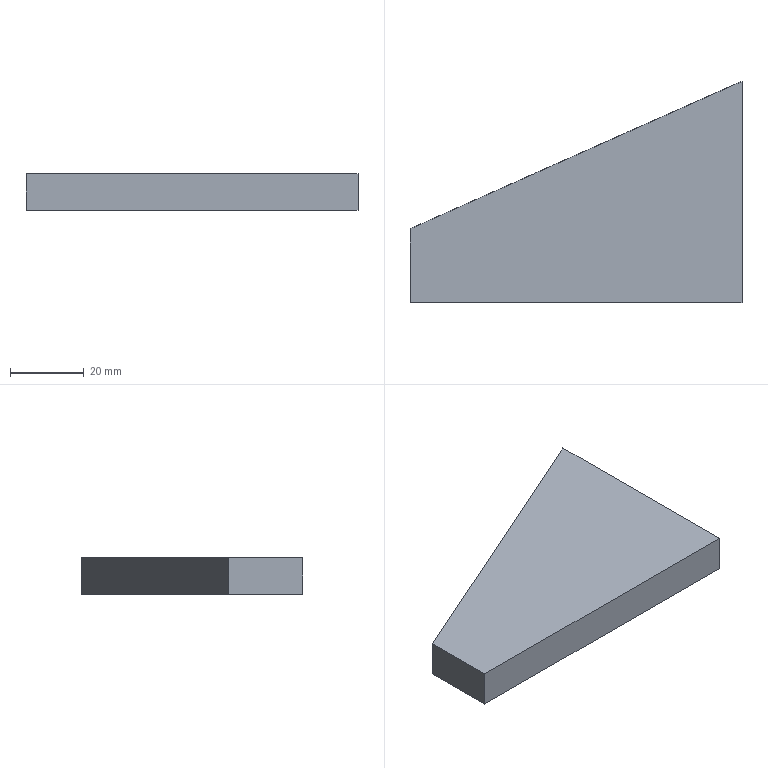Part | SolidWorks | features BaseBody 1, ICE 1 | 1 solid | 6 faces | box 90 x 60 x 10 mm | volume 36000 mm3 | plane 6
STEP:
#1=CARTESIAN_POINT('',(-25.,10.,1240.));
#2=VERTEX_POINT('',#1);
#3=CARTESIAN_POINT('',(-25.,-50.,1240.));
#4=VERTEX_POINT('',#3);
#5=CARTESIAN_POINT('',(-25.,-15.,1240.));
#6=DIRECTION('',(0.,-1.,0.));
#7=VECTOR('',#6,1000.);
#8=LINE('',#5,#7);
#9=EDGE_CURVE('',#2,#4,#8,.T.);
#10=ORIENTED_EDGE('',*,*,#9,.F.);
#11=CARTESIAN_POINT('',(-115.,-30.,1240.));
#12=VERTEX_POINT('',#11);
#13=CARTESIAN_POINT('',(-25.,10.,1240.));
#14=DIRECTION('',(-0.9138,-0.4061,0.));
#15=VECTOR('',#14,1000.);
#16=LINE('',#13,#15);
#17=EDGE_CURVE('',#2,#12,#16,.T.);
#18=ORIENTED_EDGE('',*,*,#17,.T.);
#19=CARTESIAN_POINT('',(-115.,-50.,1240.));
#20=VERTEX_POINT('',#19);
#21=CARTESIAN_POINT('',(-115.,-15.,1240.));
#22=DIRECTION('',(0.,1.,0.));
#23=VECTOR('',#22,1000.);
#24=LINE('',#21,#23);
#25=EDGE_CURVE('',#20,#12,#24,.T.);
#26=ORIENTED_EDGE('',*,*,#25,.F.);
#27=CARTESIAN_POINT('',(-70.,-50.,1240.));
#28=DIRECTION('',(-1.,0.,0.));
#29=VECTOR('',#28,1000.);
#30=LINE('',#27,#29);
#31=EDGE_CURVE('',#4,#20,#30,.T.);
#32=ORIENTED_EDGE('',*,*,#31,.F.);
#33=EDGE_LOOP('',(#10,#18,#26,#32));
#34=FACE_OUTER_BOUND('',#33,.T.);
#35=CARTESIAN_POINT('',(-23.2,-51.4,1240.));
#36=DIRECTION('',(0.,0.,-1.));
#37=DIRECTION('',(-1.,0.,0.));
#38=AXIS2_PLACEMENT_3D('',#35,#36,#37);
#39=PLANE('',#38);
#40=ADVANCED_FACE('',(#34),#39,.F.);
#41=CARTESIAN_POINT('',(-25.,10.,1230.));
#42=VERTEX_POINT('',#41);
#43=CARTESIAN_POINT('',(-25.,10.,1240.));
#44=DIRECTION('',(0.,0.,-1.));
#45=VECTOR('',#44,1000.);
#46=LINE('',#43,#45);
#47=EDGE_CURVE('',#2,#42,#46,.T.);
#48=ORIENTED_EDGE('',*,*,#47,.F.);
#49=ORIENTED_EDGE('',*,*,#9,.T.);
#50=CARTESIAN_POINT('',(-25.,-50.,1230.));
#51=VERTEX_POINT('',#50);
#52=CARTESIAN_POINT('',(-25.,-50.,1235.));
#53=DIRECTION('',(0.,0.,-1.));
#54=VECTOR('',#53,1000.);
#55=LINE('',#52,#54);
#56=EDGE_CURVE('',#4,#51,#55,.T.);
#57=ORIENTED_EDGE('',*,*,#56,.T.);
#58=CARTESIAN_POINT('',(-25.,-15.,1230.));
#59=DIRECTION('',(0.,1.,0.));
#60=VECTOR('',#59,1000.);
#61=LINE('',#58,#60);
#62=EDGE_CURVE('',#51,#42,#61,.T.);
#63=ORIENTED_EDGE('',*,*,#62,.T.);
#64=EDGE_LOOP('',(#48,#49,#57,#63));
#65=FACE_OUTER_BOUND('',#64,.T.);
#66=CARTESIAN_POINT('',(-25.,21.4,1241.145));
#67=DIRECTION('',(1.,0.,0.));
#68=DIRECTION('',(0.,-1.,0.));
#69=AXIS2_PLACEMENT_3D('',#66,#67,#68);
#70=PLANE('',#69);
#71=ADVANCED_FACE('',(#65),#70,.T.);
#72=CARTESIAN_POINT('',(-115.,-30.,1230.));
#73=VERTEX_POINT('',#72);
#74=CARTESIAN_POINT('',(-115.,-50.,1230.));
#75=VERTEX_POINT('',#74);
#76=CARTESIAN_POINT('',(-115.,-40.,1230.));
#77=DIRECTION('',(0.,-1.,0.));
#78=VECTOR('',#77,1000.);
#79=LINE('',#76,#78);
#80=EDGE_CURVE('',#73,#75,#79,.T.);
#81=ORIENTED_EDGE('',*,*,#80,.T.);
#82=CARTESIAN_POINT('',(-115.,-50.,1235.));
#83=DIRECTION('',(0.,0.,1.));
#84=VECTOR('',#83,1000.);
#85=LINE('',#82,#84);
#86=EDGE_CURVE('',#75,#20,#85,.T.);
#87=ORIENTED_EDGE('',*,*,#86,.T.);
#88=ORIENTED_EDGE('',*,*,#25,.T.);
#89=CARTESIAN_POINT('',(-115.,-30.,1235.));
#90=DIRECTION('',(0.,0.,1.));
#91=VECTOR('',#90,1000.);
#92=LINE('',#89,#91);
#93=EDGE_CURVE('',#73,#12,#92,.T.);
#94=ORIENTED_EDGE('',*,*,#93,.F.);
#95=EDGE_LOOP('',(#81,#87,#88,#94));
#96=FACE_OUTER_BOUND('',#95,.T.);
#97=CARTESIAN_POINT('',(-115.,-51.145,1241.145));
#98=DIRECTION('',(-1.,0.,0.));
#99=DIRECTION('',(0.,1.,0.));
#100=AXIS2_PLACEMENT_3D('',#97,#98,#99);
#101=PLANE('',#100);
#102=ADVANCED_FACE('',(#96),#101,.T.);
#103=CARTESIAN_POINT('',(-70.,-50.,1230.));
#104=DIRECTION('',(1.,0.,0.));
#105=VECTOR('',#104,1000.);
#106=LINE('',#103,#105);
#107=EDGE_CURVE('',#75,#51,#106,.T.);
#108=ORIENTED_EDGE('',*,*,#107,.T.);
#109=ORIENTED_EDGE('',*,*,#56,.F.);
#110=ORIENTED_EDGE('',*,*,#31,.T.);
#111=ORIENTED_EDGE('',*,*,#86,.F.);
#112=EDGE_LOOP('',(#108,#109,#110,#111));
#113=FACE_OUTER_BOUND('',#112,.T.);
#114=CARTESIAN_POINT('',(-23.2,-50.,1241.145));
#115=DIRECTION('',(0.,-1.,0.));
#116=DIRECTION('',(-1.,0.,0.));
#117=AXIS2_PLACEMENT_3D('',#114,#115,#116);
#118=PLANE('',#117);
#119=ADVANCED_FACE('',(#113),#118,.T.);
#120=CARTESIAN_POINT('',(-25.,10.,1230.));
#121=DIRECTION('',(-0.9138,-0.4061,0.));
#122=VECTOR('',#121,1000.);
#123=LINE('',#120,#122);
#124=EDGE_CURVE('',#42,#73,#123,.T.);
#125=ORIENTED_EDGE('',*,*,#124,.F.);
#126=ORIENTED_EDGE('',*,*,#62,.F.);
#127=ORIENTED_EDGE('',*,*,#107,.F.);
#128=ORIENTED_EDGE('',*,*,#80,.F.);
#129=EDGE_LOOP('',(#125,#126,#127,#128));
#130=FACE_OUTER_BOUND('',#129,.T.);
#131=CARTESIAN_POINT('',(-23.2,-51.4,1230.));
#132=DIRECTION('',(0.,0.,-1.));
#133=DIRECTION('',(-1.,0.,0.));
#134=AXIS2_PLACEMENT_3D('',#131,#132,#133);
#135=PLANE('',#134);
#136=ADVANCED_FACE('',(#130),#135,.T.);
#137=ORIENTED_EDGE('',*,*,#124,.T.);
#138=ORIENTED_EDGE('',*,*,#93,.T.);
#139=ORIENTED_EDGE('',*,*,#17,.F.);
#140=ORIENTED_EDGE('',*,*,#47,.T.);
#141=EDGE_LOOP('',(#137,#138,#139,#140));
#142=FACE_OUTER_BOUND('',#141,.T.);
#143=CARTESIAN_POINT('',(-25.,10.,1240.));
#144=DIRECTION('',(0.4061,-0.9138,0.));
#145=DIRECTION('',(0.9138,0.4061,0.));
#146=AXIS2_PLACEMENT_3D('',#143,#144,#145);
#147=PLANE('',#146);
#148=ADVANCED_FACE('',(#142),#147,.F.);
#149=CLOSED_SHELL('',(#40,#71,#102,#119,#136,#148));
#150=MANIFOLD_SOLID_BREP('',#149);
#151=CARTESIAN_POINT('',(0.,0.,0.));
#152=DIRECTION('',(0.,0.,1.));
#153=DIRECTION('',(1.,0.,0.));
#154=AXIS2_PLACEMENT_3D('',#151,#152,#153);
#155=(LENGTH_UNIT()NAMED_UNIT(*)SI_UNIT(.MILLI.,.METRE.));
#156=UNCERTAINTY_MEASURE_WITH_UNIT(LENGTH_MEASURE(0.00001),#155,'','');
#157=(NAMED_UNIT(*)PLANE_ANGLE_UNIT()SI_UNIT($,.RADIAN.));
#158=(NAMED_UNIT(*)SI_UNIT($,.STERADIAN.)SOLID_ANGLE_UNIT());
#159=(GEOMETRIC_REPRESENTATION_CONTEXT(3)GLOBAL_UNCERTAINTY_ASSIGNED_CONTEXT((#156))GLOBAL_UNIT_ASSIGNED_CONTEXT((#155,#157,#158))REPRESENTATION_CONTEXT('',''));
#160=ADVANCED_BREP_SHAPE_REPRESENTATION('',(#150,#154),#159);